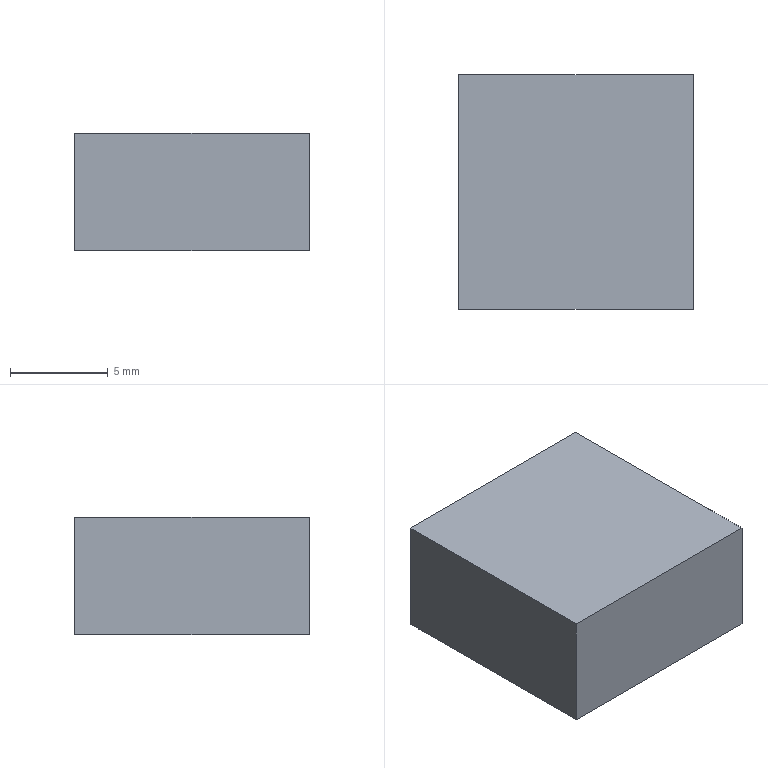Part | SolidWorks | features FlatPattern 1, SMBaseFlange 1, SheetMetal 1 | 1 solid | 6 faces | box 12 x 12 x 6 mm | volume 864 mm3 | plane 6
STEP:
#1=CARTESIAN_POINT('',(162.,350.5,0.));
#2=VERTEX_POINT('',#1);
#3=CARTESIAN_POINT('',(150.,350.5,0.));
#4=VERTEX_POINT('',#3);
#5=CARTESIAN_POINT('',(162.,350.5,0.));
#6=DIRECTION('',(-1.,0.,0.));
#7=VECTOR('',#6,1000.);
#8=LINE('',#5,#7);
#9=EDGE_CURVE('',#2,#4,#8,.T.);
#10=ORIENTED_EDGE('',*,*,#9,.T.);
#11=CARTESIAN_POINT('',(150.,350.5,6.));
#12=VERTEX_POINT('',#11);
#13=CARTESIAN_POINT('',(150.,350.5,6.));
#14=DIRECTION('',(0.,0.,-1.));
#15=VECTOR('',#14,1000.);
#16=LINE('',#13,#15);
#17=EDGE_CURVE('',#12,#4,#16,.T.);
#18=ORIENTED_EDGE('',*,*,#17,.F.);
#19=CARTESIAN_POINT('',(162.,350.5,6.));
#20=VERTEX_POINT('',#19);
#21=CARTESIAN_POINT('',(162.,350.5,6.));
#22=DIRECTION('',(-1.,0.,0.));
#23=VECTOR('',#22,1000.);
#24=LINE('',#21,#23);
#25=EDGE_CURVE('',#20,#12,#24,.T.);
#26=ORIENTED_EDGE('',*,*,#25,.F.);
#27=CARTESIAN_POINT('',(162.,350.5,6.));
#28=DIRECTION('',(0.,0.,-1.));
#29=VECTOR('',#28,1000.);
#30=LINE('',#27,#29);
#31=EDGE_CURVE('',#20,#2,#30,.T.);
#32=ORIENTED_EDGE('',*,*,#31,.T.);
#33=EDGE_LOOP('',(#10,#18,#26,#32));
#34=FACE_OUTER_BOUND('',#33,.T.);
#35=CARTESIAN_POINT('',(162.,350.5,6.));
#36=DIRECTION('',(0.,-1.,0.));
#37=DIRECTION('',(0.,0.,-1.));
#38=AXIS2_PLACEMENT_3D('',#35,#36,#37);
#39=PLANE('',#38);
#40=ADVANCED_FACE('',(#34),#39,.F.);
#41=CARTESIAN_POINT('',(150.,338.5,0.));
#42=VERTEX_POINT('',#41);
#43=CARTESIAN_POINT('',(150.,350.5,0.));
#44=DIRECTION('',(0.,-1.,0.));
#45=VECTOR('',#44,1000.);
#46=LINE('',#43,#45);
#47=EDGE_CURVE('',#4,#42,#46,.T.);
#48=ORIENTED_EDGE('',*,*,#47,.T.);
#49=CARTESIAN_POINT('',(150.,338.5,6.));
#50=VERTEX_POINT('',#49);
#51=CARTESIAN_POINT('',(150.,338.5,6.));
#52=DIRECTION('',(0.,0.,-1.));
#53=VECTOR('',#52,1000.);
#54=LINE('',#51,#53);
#55=EDGE_CURVE('',#50,#42,#54,.T.);
#56=ORIENTED_EDGE('',*,*,#55,.F.);
#57=CARTESIAN_POINT('',(150.,350.5,6.));
#58=DIRECTION('',(0.,-1.,0.));
#59=VECTOR('',#58,1000.);
#60=LINE('',#57,#59);
#61=EDGE_CURVE('',#12,#50,#60,.T.);
#62=ORIENTED_EDGE('',*,*,#61,.F.);
#63=ORIENTED_EDGE('',*,*,#17,.T.);
#64=EDGE_LOOP('',(#48,#56,#62,#63));
#65=FACE_OUTER_BOUND('',#64,.T.);
#66=CARTESIAN_POINT('',(150.,350.5,6.));
#67=DIRECTION('',(1.,0.,0.));
#68=DIRECTION('',(0.,0.,-1.));
#69=AXIS2_PLACEMENT_3D('',#66,#67,#68);
#70=PLANE('',#69);
#71=ADVANCED_FACE('',(#65),#70,.F.);
#72=CARTESIAN_POINT('',(162.,338.5,0.));
#73=VERTEX_POINT('',#72);
#74=CARTESIAN_POINT('',(150.,338.5,0.));
#75=DIRECTION('',(1.,0.,0.));
#76=VECTOR('',#75,1000.);
#77=LINE('',#74,#76);
#78=EDGE_CURVE('',#42,#73,#77,.T.);
#79=ORIENTED_EDGE('',*,*,#78,.T.);
#80=CARTESIAN_POINT('',(162.,338.5,6.));
#81=VERTEX_POINT('',#80);
#82=CARTESIAN_POINT('',(162.,338.5,6.));
#83=DIRECTION('',(0.,0.,-1.));
#84=VECTOR('',#83,1000.);
#85=LINE('',#82,#84);
#86=EDGE_CURVE('',#81,#73,#85,.T.);
#87=ORIENTED_EDGE('',*,*,#86,.F.);
#88=CARTESIAN_POINT('',(150.,338.5,6.));
#89=DIRECTION('',(1.,0.,0.));
#90=VECTOR('',#89,1000.);
#91=LINE('',#88,#90);
#92=EDGE_CURVE('',#50,#81,#91,.T.);
#93=ORIENTED_EDGE('',*,*,#92,.F.);
#94=ORIENTED_EDGE('',*,*,#55,.T.);
#95=EDGE_LOOP('',(#79,#87,#93,#94));
#96=FACE_OUTER_BOUND('',#95,.T.);
#97=CARTESIAN_POINT('',(150.,338.5,6.));
#98=DIRECTION('',(0.,1.,0.));
#99=DIRECTION('',(0.,0.,1.));
#100=AXIS2_PLACEMENT_3D('',#97,#98,#99);
#101=PLANE('',#100);
#102=ADVANCED_FACE('',(#96),#101,.F.);
#103=CARTESIAN_POINT('',(162.,338.5,0.));
#104=DIRECTION('',(0.,1.,0.));
#105=VECTOR('',#104,1000.);
#106=LINE('',#103,#105);
#107=EDGE_CURVE('',#73,#2,#106,.T.);
#108=ORIENTED_EDGE('',*,*,#107,.T.);
#109=ORIENTED_EDGE('',*,*,#31,.F.);
#110=CARTESIAN_POINT('',(162.,338.5,6.));
#111=DIRECTION('',(0.,1.,0.));
#112=VECTOR('',#111,1000.);
#113=LINE('',#110,#112);
#114=EDGE_CURVE('',#81,#20,#113,.T.);
#115=ORIENTED_EDGE('',*,*,#114,.F.);
#116=ORIENTED_EDGE('',*,*,#86,.T.);
#117=EDGE_LOOP('',(#108,#109,#115,#116));
#118=FACE_OUTER_BOUND('',#117,.T.);
#119=CARTESIAN_POINT('',(162.,338.5,6.));
#120=DIRECTION('',(-1.,0.,0.));
#121=DIRECTION('',(0.,0.,1.));
#122=AXIS2_PLACEMENT_3D('',#119,#120,#121);
#123=PLANE('',#122);
#124=ADVANCED_FACE('',(#118),#123,.F.);
#125=ORIENTED_EDGE('',*,*,#25,.T.);
#126=ORIENTED_EDGE('',*,*,#61,.T.);
#127=ORIENTED_EDGE('',*,*,#92,.T.);
#128=ORIENTED_EDGE('',*,*,#114,.T.);
#129=EDGE_LOOP('',(#125,#126,#127,#128));
#130=FACE_OUTER_BOUND('',#129,.T.);
#131=CARTESIAN_POINT('',(0.,0.,6.));
#132=DIRECTION('',(0.,0.,1.));
#133=DIRECTION('',(1.,0.,0.));
#134=AXIS2_PLACEMENT_3D('',#131,#132,#133);
#135=PLANE('',#134);
#136=ADVANCED_FACE('',(#130),#135,.T.);
#137=ORIENTED_EDGE('',*,*,#9,.F.);
#138=ORIENTED_EDGE('',*,*,#107,.F.);
#139=ORIENTED_EDGE('',*,*,#78,.F.);
#140=ORIENTED_EDGE('',*,*,#47,.F.);
#141=EDGE_LOOP('',(#137,#138,#139,#140));
#142=FACE_OUTER_BOUND('',#141,.T.);
#143=CARTESIAN_POINT('',(0.,0.,0.));
#144=DIRECTION('',(0.,0.,1.));
#145=DIRECTION('',(1.,0.,0.));
#146=AXIS2_PLACEMENT_3D('',#143,#144,#145);
#147=PLANE('',#146);
#148=ADVANCED_FACE('',(#142),#147,.F.);
#149=CLOSED_SHELL('',(#40,#71,#102,#124,#136,#148));
#150=MANIFOLD_SOLID_BREP('',#149);
#151=CARTESIAN_POINT('',(0.,0.,0.));
#152=DIRECTION('',(0.,0.,1.));
#153=DIRECTION('',(1.,0.,0.));
#154=AXIS2_PLACEMENT_3D('',#151,#152,#153);
#155=(LENGTH_UNIT()NAMED_UNIT(*)SI_UNIT(.MILLI.,.METRE.));
#156=UNCERTAINTY_MEASURE_WITH_UNIT(LENGTH_MEASURE(0.00001),#155,'','');
#157=(NAMED_UNIT(*)PLANE_ANGLE_UNIT()SI_UNIT($,.RADIAN.));
#158=(NAMED_UNIT(*)SI_UNIT($,.STERADIAN.)SOLID_ANGLE_UNIT());
#159=(GEOMETRIC_REPRESENTATION_CONTEXT(3)GLOBAL_UNCERTAINTY_ASSIGNED_CONTEXT((#156))GLOBAL_UNIT_ASSIGNED_CONTEXT((#155,#157,#158))REPRESENTATION_CONTEXT('',''));
#160=ADVANCED_BREP_SHAPE_REPRESENTATION('',(#150,#154),#159);